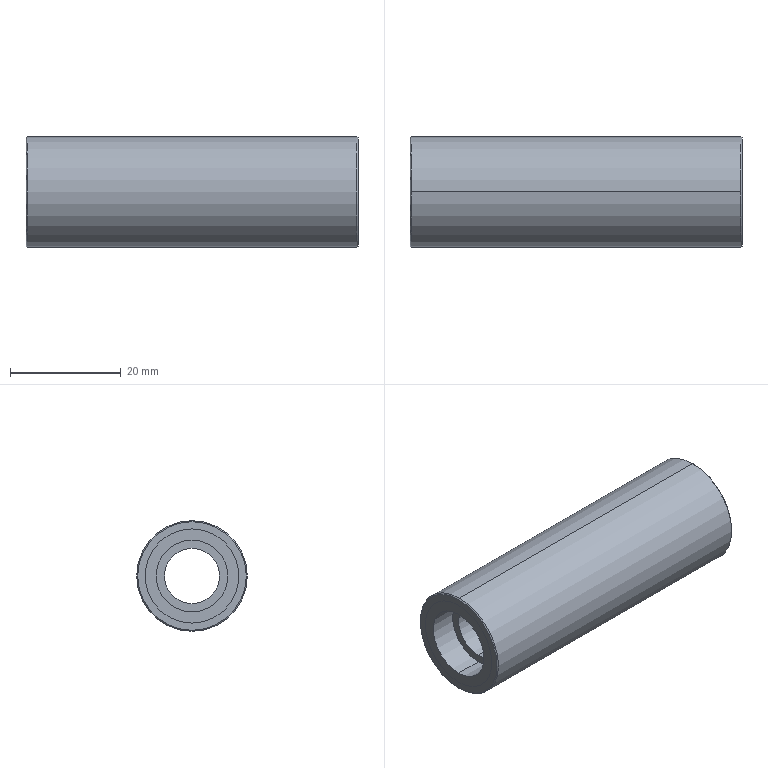Part | SolidWorks | features Chamfer 1, ICE 1, Revolution 1 | 2 solids | 22 faces | box 60 x 20 x 20 mm | volume 13593 mm3 | cylinder 12 | plane 6 | cone 4 | commonest cylinder face diameters 13 x4 17 x4 10 x2 20 x2
STEP:
#1=CARTESIAN_POINT('',(5.,0.,-6.5));
#2=VERTEX_POINT('',#1);
#3=CARTESIAN_POINT('',(5.,0.,6.5));
#4=VERTEX_POINT('',#3);
#5=CARTESIAN_POINT('',(5.,0.,0.));
#6=DIRECTION('',(-1.,0.,0.));
#7=DIRECTION('',(0.,0.,1.));
#8=AXIS2_PLACEMENT_3D('',#5,#6,#7);
#9=CIRCLE('',#8,6.5);
#10=EDGE_CURVE('',#2,#4,#9,.T.);
#11=ORIENTED_EDGE('',*,*,#10,.F.);
#12=CARTESIAN_POINT('',(0.,0.,-6.5));
#13=VERTEX_POINT('',#12);
#14=CARTESIAN_POINT('',(0.,0.,-6.5));
#15=DIRECTION('',(-1.,0.,0.));
#16=VECTOR('',#15,1000.);
#17=LINE('',#14,#16);
#18=EDGE_CURVE('',#2,#13,#17,.T.);
#19=ORIENTED_EDGE('',*,*,#18,.T.);
#20=CARTESIAN_POINT('',(0.,0.,6.5));
#21=VERTEX_POINT('',#20);
#22=CARTESIAN_POINT('',(0.,0.,0.));
#23=DIRECTION('',(-1.,0.,0.));
#24=DIRECTION('',(0.,0.,1.));
#25=AXIS2_PLACEMENT_3D('',#22,#23,#24);
#26=CIRCLE('',#25,6.5);
#27=EDGE_CURVE('',#13,#21,#26,.T.);
#28=ORIENTED_EDGE('',*,*,#27,.T.);
#29=CARTESIAN_POINT('',(0.,0.,6.5));
#30=DIRECTION('',(-1.,0.,0.));
#31=VECTOR('',#30,1000.);
#32=LINE('',#29,#31);
#33=EDGE_CURVE('',#4,#21,#32,.T.);
#34=ORIENTED_EDGE('',*,*,#33,.F.);
#35=EDGE_LOOP('',(#11,#19,#28,#34));
#36=FACE_OUTER_BOUND('',#35,.T.);
#37=CARTESIAN_POINT('',(0.,0.,0.));
#38=DIRECTION('',(-1.,0.,0.));
#39=DIRECTION('',(0.,0.,1.));
#40=AXIS2_PLACEMENT_3D('',#37,#38,#39);
#41=CYLINDRICAL_SURFACE('',#40,6.5);
#42=ADVANCED_FACE('',(#36),#41,.F.);
#43=CARTESIAN_POINT('',(55.,0.,-5.));
#44=VERTEX_POINT('',#43);
#45=CARTESIAN_POINT('',(55.,0.,5.));
#46=VERTEX_POINT('',#45);
#47=CARTESIAN_POINT('',(55.,0.,0.));
#48=DIRECTION('',(-1.,0.,0.));
#49=DIRECTION('',(0.,0.,1.));
#50=AXIS2_PLACEMENT_3D('',#47,#48,#49);
#51=CIRCLE('',#50,5.);
#52=EDGE_CURVE('',#44,#46,#51,.T.);
#53=ORIENTED_EDGE('',*,*,#52,.F.);
#54=CARTESIAN_POINT('',(5.,0.,-5.));
#55=VERTEX_POINT('',#54);
#56=CARTESIAN_POINT('',(0.,0.,-5.));
#57=DIRECTION('',(-1.,0.,0.));
#58=VECTOR('',#57,1000.);
#59=LINE('',#56,#58);
#60=EDGE_CURVE('',#44,#55,#59,.T.);
#61=ORIENTED_EDGE('',*,*,#60,.T.);
#62=CARTESIAN_POINT('',(5.,0.,5.));
#63=VERTEX_POINT('',#62);
#64=CARTESIAN_POINT('',(5.,0.,0.));
#65=DIRECTION('',(-1.,0.,0.));
#66=DIRECTION('',(0.,0.,1.));
#67=AXIS2_PLACEMENT_3D('',#64,#65,#66);
#68=CIRCLE('',#67,5.);
#69=EDGE_CURVE('',#55,#63,#68,.T.);
#70=ORIENTED_EDGE('',*,*,#69,.T.);
#71=CARTESIAN_POINT('',(0.,0.,5.));
#72=DIRECTION('',(-1.,0.,0.));
#73=VECTOR('',#72,1000.);
#74=LINE('',#71,#73);
#75=EDGE_CURVE('',#46,#63,#74,.T.);
#76=ORIENTED_EDGE('',*,*,#75,.F.);
#77=EDGE_LOOP('',(#53,#61,#70,#76));
#78=FACE_OUTER_BOUND('',#77,.T.);
#79=CARTESIAN_POINT('',(0.,0.,0.));
#80=DIRECTION('',(-1.,0.,0.));
#81=DIRECTION('',(0.,0.,1.));
#82=AXIS2_PLACEMENT_3D('',#79,#80,#81);
#83=CYLINDRICAL_SURFACE('',#82,5.);
#84=ADVANCED_FACE('',(#78),#83,.F.);
#85=CARTESIAN_POINT('',(60.,0.,-6.5));
#86=VERTEX_POINT('',#85);
#87=CARTESIAN_POINT('',(60.,0.,6.5));
#88=VERTEX_POINT('',#87);
#89=CARTESIAN_POINT('',(60.,0.,0.));
#90=DIRECTION('',(-1.,0.,0.));
#91=DIRECTION('',(0.,0.,1.));
#92=AXIS2_PLACEMENT_3D('',#89,#90,#91);
#93=CIRCLE('',#92,6.5);
#94=EDGE_CURVE('',#86,#88,#93,.T.);
#95=ORIENTED_EDGE('',*,*,#94,.F.);
#96=CARTESIAN_POINT('',(55.,0.,-6.5));
#97=VERTEX_POINT('',#96);
#98=CARTESIAN_POINT('',(0.,0.,-6.5));
#99=DIRECTION('',(-1.,0.,0.));
#100=VECTOR('',#99,1000.);
#101=LINE('',#98,#100);
#102=EDGE_CURVE('',#86,#97,#101,.T.);
#103=ORIENTED_EDGE('',*,*,#102,.T.);
#104=CARTESIAN_POINT('',(55.,0.,6.5));
#105=VERTEX_POINT('',#104);
#106=CARTESIAN_POINT('',(55.,0.,0.));
#107=DIRECTION('',(-1.,0.,0.));
#108=DIRECTION('',(0.,0.,1.));
#109=AXIS2_PLACEMENT_3D('',#106,#107,#108);
#110=CIRCLE('',#109,6.5);
#111=EDGE_CURVE('',#97,#105,#110,.T.);
#112=ORIENTED_EDGE('',*,*,#111,.T.);
#113=CARTESIAN_POINT('',(0.,0.,6.5));
#114=DIRECTION('',(-1.,0.,0.));
#115=VECTOR('',#114,1000.);
#116=LINE('',#113,#115);
#117=EDGE_CURVE('',#88,#105,#116,.T.);
#118=ORIENTED_EDGE('',*,*,#117,.F.);
#119=EDGE_LOOP('',(#95,#103,#112,#118));
#120=FACE_OUTER_BOUND('',#119,.T.);
#121=CARTESIAN_POINT('',(0.,0.,0.));
#122=DIRECTION('',(-1.,0.,0.));
#123=DIRECTION('',(0.,0.,1.));
#124=AXIS2_PLACEMENT_3D('',#121,#122,#123);
#125=CYLINDRICAL_SURFACE('',#124,6.5);
#126=ADVANCED_FACE('',(#120),#125,.F.);
#127=CARTESIAN_POINT('',(60.,0.,8.5));
#128=VERTEX_POINT('',#127);
#129=CARTESIAN_POINT('',(60.,0.,-8.5));
#130=VERTEX_POINT('',#129);
#131=CARTESIAN_POINT('',(60.,0.,0.));
#132=DIRECTION('',(-1.,0.,0.));
#133=DIRECTION('',(0.,0.,1.));
#134=AXIS2_PLACEMENT_3D('',#131,#132,#133);
#135=CIRCLE('',#134,8.5);
#136=EDGE_CURVE('',#128,#130,#135,.T.);
#137=ORIENTED_EDGE('',*,*,#136,.T.);
#138=CARTESIAN_POINT('',(0.,0.,-8.5));
#139=VERTEX_POINT('',#138);
#140=CARTESIAN_POINT('',(0.,0.,-8.5));
#141=DIRECTION('',(-1.,0.,0.));
#142=VECTOR('',#141,1000.);
#143=LINE('',#140,#142);
#144=EDGE_CURVE('',#130,#139,#143,.T.);
#145=ORIENTED_EDGE('',*,*,#144,.T.);
#146=CARTESIAN_POINT('',(0.,0.,8.5));
#147=VERTEX_POINT('',#146);
#148=CARTESIAN_POINT('',(0.,0.,0.));
#149=DIRECTION('',(-1.,0.,0.));
#150=DIRECTION('',(0.,0.,1.));
#151=AXIS2_PLACEMENT_3D('',#148,#149,#150);
#152=CIRCLE('',#151,8.5);
#153=EDGE_CURVE('',#147,#139,#152,.T.);
#154=ORIENTED_EDGE('',*,*,#153,.F.);
#155=CARTESIAN_POINT('',(0.,0.,8.5));
#156=DIRECTION('',(-1.,0.,0.));
#157=VECTOR('',#156,1000.);
#158=LINE('',#155,#157);
#159=EDGE_CURVE('',#128,#147,#158,.T.);
#160=ORIENTED_EDGE('',*,*,#159,.F.);
#161=EDGE_LOOP('',(#137,#145,#154,#160));
#162=FACE_OUTER_BOUND('',#161,.T.);
#163=CARTESIAN_POINT('',(0.,0.,0.));
#164=DIRECTION('',(-1.,0.,0.));
#165=DIRECTION('',(0.,0.,1.));
#166=AXIS2_PLACEMENT_3D('',#163,#164,#165);
#167=CYLINDRICAL_SURFACE('',#166,8.5);
#168=ADVANCED_FACE('',(#162),#167,.T.);
#169=CARTESIAN_POINT('',(0.,0.,0.));
#170=DIRECTION('',(-1.,0.,0.));
#171=DIRECTION('',(0.,0.,1.));
#172=AXIS2_PLACEMENT_3D('',#169,#170,#171);
#173=CIRCLE('',#172,6.5);
#174=EDGE_CURVE('',#21,#13,#173,.T.);
#175=ORIENTED_EDGE('',*,*,#174,.F.);
#176=ORIENTED_EDGE('',*,*,#27,.F.);
#177=EDGE_LOOP('',(#175,#176));
#178=FACE_BOUND('',#177,.T.);
#179=ORIENTED_EDGE('',*,*,#153,.T.);
#180=CARTESIAN_POINT('',(0.,0.,0.));
#181=DIRECTION('',(-1.,0.,0.));
#182=DIRECTION('',(0.,0.,1.));
#183=AXIS2_PLACEMENT_3D('',#180,#181,#182);
#184=CIRCLE('',#183,8.5);
#185=EDGE_CURVE('',#139,#147,#184,.T.);
#186=ORIENTED_EDGE('',*,*,#185,.T.);
#187=EDGE_LOOP('',(#179,#186));
#188=FACE_OUTER_BOUND('',#187,.T.);
#189=CARTESIAN_POINT('',(0.,6.5,0.));
#190=DIRECTION('',(1.,0.,0.));
#191=DIRECTION('',(0.,0.,-1.));
#192=AXIS2_PLACEMENT_3D('',#189,#190,#191);
#193=PLANE('',#192);
#194=ADVANCED_FACE('',(#178,#188),#193,.F.);
#195=ORIENTED_EDGE('',*,*,#144,.F.);
#196=CARTESIAN_POINT('',(60.,0.,0.));
#197=DIRECTION('',(-1.,0.,0.));
#198=DIRECTION('',(0.,0.,1.));
#199=AXIS2_PLACEMENT_3D('',#196,#197,#198);
#200=CIRCLE('',#199,8.5);
#201=EDGE_CURVE('',#130,#128,#200,.T.);
#202=ORIENTED_EDGE('',*,*,#201,.T.);
#203=ORIENTED_EDGE('',*,*,#159,.T.);
#204=ORIENTED_EDGE('',*,*,#185,.F.);
#205=EDGE_LOOP('',(#195,#202,#203,#204));
#206=FACE_OUTER_BOUND('',#205,.T.);
#207=CARTESIAN_POINT('',(0.,0.,0.));
#208=DIRECTION('',(-1.,0.,0.));
#209=DIRECTION('',(0.,0.,1.));
#210=AXIS2_PLACEMENT_3D('',#207,#208,#209);
#211=CYLINDRICAL_SURFACE('',#210,8.5);
#212=ADVANCED_FACE('',(#206),#211,.T.);
#213=ORIENTED_EDGE('',*,*,#136,.F.);
#214=ORIENTED_EDGE('',*,*,#201,.F.);
#215=EDGE_LOOP('',(#213,#214));
#216=FACE_OUTER_BOUND('',#215,.T.);
#217=CARTESIAN_POINT('',(60.,0.,0.));
#218=DIRECTION('',(-1.,0.,0.));
#219=DIRECTION('',(0.,0.,1.));
#220=AXIS2_PLACEMENT_3D('',#217,#218,#219);
#221=CIRCLE('',#220,6.5);
#222=EDGE_CURVE('',#88,#86,#221,.T.);
#223=ORIENTED_EDGE('',*,*,#222,.T.);
#224=ORIENTED_EDGE('',*,*,#94,.T.);
#225=EDGE_LOOP('',(#223,#224));
#226=FACE_BOUND('',#225,.T.);
#227=CARTESIAN_POINT('',(60.,8.5,0.));
#228=DIRECTION('',(-1.,0.,0.));
#229=DIRECTION('',(0.,0.,1.));
#230=AXIS2_PLACEMENT_3D('',#227,#228,#229);
#231=PLANE('',#230);
#232=ADVANCED_FACE('',(#216,#226),#231,.F.);
#233=ORIENTED_EDGE('',*,*,#102,.F.);
#234=ORIENTED_EDGE('',*,*,#222,.F.);
#235=ORIENTED_EDGE('',*,*,#117,.T.);
#236=CARTESIAN_POINT('',(55.,0.,0.));
#237=DIRECTION('',(-1.,0.,0.));
#238=DIRECTION('',(0.,0.,1.));
#239=AXIS2_PLACEMENT_3D('',#236,#237,#238);
#240=CIRCLE('',#239,6.5);
#241=EDGE_CURVE('',#105,#97,#240,.T.);
#242=ORIENTED_EDGE('',*,*,#241,.T.);
#243=EDGE_LOOP('',(#233,#234,#235,#242));
#244=FACE_OUTER_BOUND('',#243,.T.);
#245=CARTESIAN_POINT('',(0.,0.,0.));
#246=DIRECTION('',(-1.,0.,0.));
#247=DIRECTION('',(0.,0.,1.));
#248=AXIS2_PLACEMENT_3D('',#245,#246,#247);
#249=CYLINDRICAL_SURFACE('',#248,6.5);
#250=ADVANCED_FACE('',(#244),#249,.F.);
#251=ORIENTED_EDGE('',*,*,#241,.F.);
#252=ORIENTED_EDGE('',*,*,#111,.F.);
#253=EDGE_LOOP('',(#251,#252));
#254=FACE_OUTER_BOUND('',#253,.T.);
#255=CARTESIAN_POINT('',(55.,0.,0.));
#256=DIRECTION('',(-1.,0.,0.));
#257=DIRECTION('',(0.,0.,1.));
#258=AXIS2_PLACEMENT_3D('',#255,#256,#257);
#259=CIRCLE('',#258,5.);
#260=EDGE_CURVE('',#46,#44,#259,.T.);
#261=ORIENTED_EDGE('',*,*,#260,.T.);
#262=ORIENTED_EDGE('',*,*,#52,.T.);
#263=EDGE_LOOP('',(#261,#262));
#264=FACE_BOUND('',#263,.T.);
#265=CARTESIAN_POINT('',(55.,6.5,0.));
#266=DIRECTION('',(-1.,0.,0.));
#267=DIRECTION('',(0.,0.,1.));
#268=AXIS2_PLACEMENT_3D('',#265,#266,#267);
#269=PLANE('',#268);
#270=ADVANCED_FACE('',(#254,#264),#269,.F.);
#271=ORIENTED_EDGE('',*,*,#60,.F.);
#272=ORIENTED_EDGE('',*,*,#260,.F.);
#273=ORIENTED_EDGE('',*,*,#75,.T.);
#274=CARTESIAN_POINT('',(5.,0.,0.));
#275=DIRECTION('',(-1.,0.,0.));
#276=DIRECTION('',(0.,0.,1.));
#277=AXIS2_PLACEMENT_3D('',#274,#275,#276);
#278=CIRCLE('',#277,5.);
#279=EDGE_CURVE('',#63,#55,#278,.T.);
#280=ORIENTED_EDGE('',*,*,#279,.T.);
#281=EDGE_LOOP('',(#271,#272,#273,#280));
#282=FACE_OUTER_BOUND('',#281,.T.);
#283=CARTESIAN_POINT('',(0.,0.,0.));
#284=DIRECTION('',(-1.,0.,0.));
#285=DIRECTION('',(0.,0.,1.));
#286=AXIS2_PLACEMENT_3D('',#283,#284,#285);
#287=CYLINDRICAL_SURFACE('',#286,5.);
#288=ADVANCED_FACE('',(#282),#287,.F.);
#289=ORIENTED_EDGE('',*,*,#279,.F.);
#290=ORIENTED_EDGE('',*,*,#69,.F.);
#291=EDGE_LOOP('',(#289,#290));
#292=FACE_BOUND('',#291,.T.);
#293=CARTESIAN_POINT('',(5.,0.,0.));
#294=DIRECTION('',(-1.,0.,0.));
#295=DIRECTION('',(0.,0.,1.));
#296=AXIS2_PLACEMENT_3D('',#293,#294,#295);
#297=CIRCLE('',#296,6.5);
#298=EDGE_CURVE('',#4,#2,#297,.T.);
#299=ORIENTED_EDGE('',*,*,#298,.T.);
#300=ORIENTED_EDGE('',*,*,#10,.T.);
#301=EDGE_LOOP('',(#299,#300));
#302=FACE_OUTER_BOUND('',#301,.T.);
#303=CARTESIAN_POINT('',(5.,5.,0.));
#304=DIRECTION('',(1.,0.,0.));
#305=DIRECTION('',(0.,0.,-1.));
#306=AXIS2_PLACEMENT_3D('',#303,#304,#305);
#307=PLANE('',#306);
#308=ADVANCED_FACE('',(#292,#302),#307,.F.);
#309=ORIENTED_EDGE('',*,*,#18,.F.);
#310=ORIENTED_EDGE('',*,*,#298,.F.);
#311=ORIENTED_EDGE('',*,*,#33,.T.);
#312=ORIENTED_EDGE('',*,*,#174,.T.);
#313=EDGE_LOOP('',(#309,#310,#311,#312));
#314=FACE_OUTER_BOUND('',#313,.T.);
#315=CARTESIAN_POINT('',(0.,0.,0.));
#316=DIRECTION('',(-1.,0.,0.));
#317=DIRECTION('',(0.,0.,1.));
#318=AXIS2_PLACEMENT_3D('',#315,#316,#317);
#319=CYLINDRICAL_SURFACE('',#318,6.5);
#320=ADVANCED_FACE('',(#314),#319,.F.);
#321=CLOSED_SHELL('',(#42,#84,#126,#168,#194,#212,#232,#250,#270,#288,#308,#320));
#322=MANIFOLD_SOLID_BREP('',#321);
#323=CARTESIAN_POINT('',(60.,0.,-9.8));
#324=VERTEX_POINT('',#323);
#325=CARTESIAN_POINT('',(60.,0.,9.8));
#326=VERTEX_POINT('',#325);
#327=CARTESIAN_POINT('',(60.,0.,0.));
#328=DIRECTION('',(1.,0.,0.));
#329=DIRECTION('',(0.,0.,-1.));
#330=AXIS2_PLACEMENT_3D('',#327,#328,#329);
#331=CIRCLE('',#330,9.8);
#332=EDGE_CURVE('',#324,#326,#331,.T.);
#333=ORIENTED_EDGE('',*,*,#332,.F.);
#334=CARTESIAN_POINT('',(59.8,0.,-10.));
#335=VERTEX_POINT('',#334);
#336=CARTESIAN_POINT('',(60.,0.,-9.8));
#337=DIRECTION('',(-0.7071,0.,-0.7071));
#338=VECTOR('',#337,1000.);
#339=LINE('',#336,#338);
#340=EDGE_CURVE('',#324,#335,#339,.T.);
#341=ORIENTED_EDGE('',*,*,#340,.T.);
#342=CARTESIAN_POINT('',(59.8,0.,10.));
#343=VERTEX_POINT('',#342);
#344=CARTESIAN_POINT('',(59.8,0.,0.));
#345=DIRECTION('',(-1.,0.,0.));
#346=DIRECTION('',(0.,0.,-1.));
#347=AXIS2_PLACEMENT_3D('',#344,#345,#346);
#348=CIRCLE('',#347,10.);
#349=EDGE_CURVE('',#343,#335,#348,.T.);
#350=ORIENTED_EDGE('',*,*,#349,.F.);
#351=CARTESIAN_POINT('',(60.,0.,9.8));
#352=DIRECTION('',(-0.7071,0.,0.7071));
#353=VECTOR('',#352,1000.);
#354=LINE('',#351,#353);
#355=EDGE_CURVE('',#326,#343,#354,.T.);
#356=ORIENTED_EDGE('',*,*,#355,.F.);
#357=EDGE_LOOP('',(#333,#341,#350,#356));
#358=FACE_OUTER_BOUND('',#357,.T.);
#359=CARTESIAN_POINT('',(60.,0.,0.));
#360=DIRECTION('',(-1.,0.,0.));
#361=DIRECTION('',(0.,0.,1.));
#362=AXIS2_PLACEMENT_3D('',#359,#360,#361);
#363=CONICAL_SURFACE('',#362,9.8,0.7854);
#364=ADVANCED_FACE('',(#358),#363,.T.);
#365=CARTESIAN_POINT('',(0.,0.,9.8));
#366=VERTEX_POINT('',#365);
#367=CARTESIAN_POINT('',(0.,0.,-9.8));
#368=VERTEX_POINT('',#367);
#369=CARTESIAN_POINT('',(0.,0.,0.));
#370=DIRECTION('',(-1.,0.,0.));
#371=DIRECTION('',(0.,0.,-1.));
#372=AXIS2_PLACEMENT_3D('',#369,#370,#371);
#373=CIRCLE('',#372,9.8);
#374=EDGE_CURVE('',#366,#368,#373,.T.);
#375=ORIENTED_EDGE('',*,*,#374,.F.);
#376=CARTESIAN_POINT('',(0.2,0.,10.));
#377=VERTEX_POINT('',#376);
#378=CARTESIAN_POINT('',(0.,0.,9.8));
#379=DIRECTION('',(0.7071,0.,0.7071));
#380=VECTOR('',#379,1000.);
#381=LINE('',#378,#380);
#382=EDGE_CURVE('',#366,#377,#381,.T.);
#383=ORIENTED_EDGE('',*,*,#382,.T.);
#384=CARTESIAN_POINT('',(0.2,0.,-10.));
#385=VERTEX_POINT('',#384);
#386=CARTESIAN_POINT('',(0.2,0.,0.));
#387=DIRECTION('',(1.,0.,0.));
#388=DIRECTION('',(0.,0.,-1.));
#389=AXIS2_PLACEMENT_3D('',#386,#387,#388);
#390=CIRCLE('',#389,10.);
#391=EDGE_CURVE('',#385,#377,#390,.T.);
#392=ORIENTED_EDGE('',*,*,#391,.F.);
#393=CARTESIAN_POINT('',(0.,0.,-9.8));
#394=DIRECTION('',(0.7071,0.,-0.7071));
#395=VECTOR('',#394,1000.);
#396=LINE('',#393,#395);
#397=EDGE_CURVE('',#368,#385,#396,.T.);
#398=ORIENTED_EDGE('',*,*,#397,.F.);
#399=EDGE_LOOP('',(#375,#383,#392,#398));
#400=FACE_OUTER_BOUND('',#399,.T.);
#401=CARTESIAN_POINT('',(0.,0.,0.));
#402=DIRECTION('',(1.,0.,0.));
#403=DIRECTION('',(0.,0.,-1.));
#404=AXIS2_PLACEMENT_3D('',#401,#402,#403);
#405=CONICAL_SURFACE('',#404,9.8,0.7854);
#406=ADVANCED_FACE('',(#400),#405,.T.);
#407=CARTESIAN_POINT('',(0.,0.,-8.5));
#408=VERTEX_POINT('',#407);
#409=CARTESIAN_POINT('',(0.,0.,8.5));
#410=VERTEX_POINT('',#409);
#411=CARTESIAN_POINT('',(0.,0.,0.));
#412=DIRECTION('',(-1.,0.,0.));
#413=DIRECTION('',(0.,0.,-1.));
#414=AXIS2_PLACEMENT_3D('',#411,#412,#413);
#415=CIRCLE('',#414,8.5);
#416=EDGE_CURVE('',#408,#410,#415,.T.);
#417=ORIENTED_EDGE('',*,*,#416,.T.);
#418=CARTESIAN_POINT('',(60.,0.,8.5));
#419=VERTEX_POINT('',#418);
#420=CARTESIAN_POINT('',(-28.284,0.,8.5));
#421=DIRECTION('',(1.,0.,0.));
#422=VECTOR('',#421,1000.);
#423=LINE('',#420,#422);
#424=EDGE_CURVE('',#410,#419,#423,.T.);
#425=ORIENTED_EDGE('',*,*,#424,.T.);
#426=CARTESIAN_POINT('',(60.,0.,-8.5));
#427=VERTEX_POINT('',#426);
#428=CARTESIAN_POINT('',(60.,0.,0.));
#429=DIRECTION('',(1.,0.,0.));
#430=DIRECTION('',(0.,0.,-1.));
#431=AXIS2_PLACEMENT_3D('',#428,#429,#430);
#432=CIRCLE('',#431,8.5);
#433=EDGE_CURVE('',#419,#427,#432,.T.);
#434=ORIENTED_EDGE('',*,*,#433,.T.);
#435=CARTESIAN_POINT('',(-28.284,0.,-8.5));
#436=DIRECTION('',(1.,0.,0.));
#437=VECTOR('',#436,1000.);
#438=LINE('',#435,#437);
#439=EDGE_CURVE('',#408,#427,#438,.T.);
#440=ORIENTED_EDGE('',*,*,#439,.F.);
#441=EDGE_LOOP('',(#417,#425,#434,#440));
#442=FACE_OUTER_BOUND('',#441,.T.);
#443=CARTESIAN_POINT('',(-28.284,0.,0.));
#444=DIRECTION('',(1.,0.,0.));
#445=DIRECTION('',(0.,0.,-1.));
#446=AXIS2_PLACEMENT_3D('',#443,#444,#445);
#447=CYLINDRICAL_SURFACE('',#446,8.5);
#448=ADVANCED_FACE('',(#442),#447,.F.);
#449=ORIENTED_EDGE('',*,*,#391,.T.);
#450=CARTESIAN_POINT('',(-28.284,0.,10.));
#451=DIRECTION('',(1.,0.,0.));
#452=VECTOR('',#451,1000.);
#453=LINE('',#450,#452);
#454=EDGE_CURVE('',#377,#343,#453,.T.);
#455=ORIENTED_EDGE('',*,*,#454,.T.);
#456=ORIENTED_EDGE('',*,*,#349,.T.);
#457=CARTESIAN_POINT('',(-28.284,0.,-10.));
#458=DIRECTION('',(1.,0.,0.));
#459=VECTOR('',#458,1000.);
#460=LINE('',#457,#459);
#461=EDGE_CURVE('',#385,#335,#460,.T.);
#462=ORIENTED_EDGE('',*,*,#461,.F.);
#463=EDGE_LOOP('',(#449,#455,#456,#462));
#464=FACE_OUTER_BOUND('',#463,.T.);
#465=CARTESIAN_POINT('',(-28.284,0.,0.));
#466=DIRECTION('',(1.,0.,0.));
#467=DIRECTION('',(0.,0.,-1.));
#468=AXIS2_PLACEMENT_3D('',#465,#466,#467);
#469=CYLINDRICAL_SURFACE('',#468,10.);
#470=ADVANCED_FACE('',(#464),#469,.T.);
#471=ORIENTED_EDGE('',*,*,#454,.F.);
#472=CARTESIAN_POINT('',(0.2,0.,0.));
#473=DIRECTION('',(1.,0.,0.));
#474=DIRECTION('',(0.,0.,-1.));
#475=AXIS2_PLACEMENT_3D('',#472,#473,#474);
#476=CIRCLE('',#475,10.);
#477=EDGE_CURVE('',#377,#385,#476,.T.);
#478=ORIENTED_EDGE('',*,*,#477,.T.);
#479=ORIENTED_EDGE('',*,*,#461,.T.);
#480=CARTESIAN_POINT('',(59.8,0.,0.));
#481=DIRECTION('',(-1.,0.,0.));
#482=DIRECTION('',(0.,0.,-1.));
#483=AXIS2_PLACEMENT_3D('',#480,#481,#482);
#484=CIRCLE('',#483,10.);
#485=EDGE_CURVE('',#335,#343,#484,.T.);
#486=ORIENTED_EDGE('',*,*,#485,.T.);
#487=EDGE_LOOP('',(#471,#478,#479,#486));
#488=FACE_OUTER_BOUND('',#487,.T.);
#489=CARTESIAN_POINT('',(-28.284,0.,0.));
#490=DIRECTION('',(1.,0.,0.));
#491=DIRECTION('',(0.,0.,-1.));
#492=AXIS2_PLACEMENT_3D('',#489,#490,#491);
#493=CYLINDRICAL_SURFACE('',#492,10.);
#494=ADVANCED_FACE('',(#488),#493,.T.);
#495=CARTESIAN_POINT('',(60.,0.,0.));
#496=DIRECTION('',(1.,0.,0.));
#497=DIRECTION('',(0.,0.,-1.));
#498=AXIS2_PLACEMENT_3D('',#495,#496,#497);
#499=CIRCLE('',#498,9.8);
#500=EDGE_CURVE('',#326,#324,#499,.T.);
#501=ORIENTED_EDGE('',*,*,#500,.T.);
#502=ORIENTED_EDGE('',*,*,#332,.T.);
#503=EDGE_LOOP('',(#501,#502));
#504=FACE_OUTER_BOUND('',#503,.T.);
#505=CARTESIAN_POINT('',(60.,0.,0.));
#506=DIRECTION('',(1.,0.,0.));
#507=DIRECTION('',(0.,0.,-1.));
#508=AXIS2_PLACEMENT_3D('',#505,#506,#507);
#509=CIRCLE('',#508,8.5);
#510=EDGE_CURVE('',#427,#419,#509,.T.);
#511=ORIENTED_EDGE('',*,*,#510,.F.);
#512=ORIENTED_EDGE('',*,*,#433,.F.);
#513=EDGE_LOOP('',(#511,#512));
#514=FACE_BOUND('',#513,.T.);
#515=CARTESIAN_POINT('',(60.,0.,0.));
#516=DIRECTION('',(1.,0.,0.));
#517=DIRECTION('',(0.,0.,-1.));
#518=AXIS2_PLACEMENT_3D('',#515,#516,#517);
#519=PLANE('',#518);
#520=ADVANCED_FACE('',(#504,#514),#519,.T.);
#521=ORIENTED_EDGE('',*,*,#424,.F.);
#522=CARTESIAN_POINT('',(0.,0.,0.));
#523=DIRECTION('',(-1.,0.,0.));
#524=DIRECTION('',(0.,0.,-1.));
#525=AXIS2_PLACEMENT_3D('',#522,#523,#524);
#526=CIRCLE('',#525,8.5);
#527=EDGE_CURVE('',#410,#408,#526,.T.);
#528=ORIENTED_EDGE('',*,*,#527,.T.);
#529=ORIENTED_EDGE('',*,*,#439,.T.);
#530=ORIENTED_EDGE('',*,*,#510,.T.);
#531=EDGE_LOOP('',(#521,#528,#529,#530));
#532=FACE_OUTER_BOUND('',#531,.T.);
#533=CARTESIAN_POINT('',(-28.284,0.,0.));
#534=DIRECTION('',(1.,0.,0.));
#535=DIRECTION('',(0.,0.,-1.));
#536=AXIS2_PLACEMENT_3D('',#533,#534,#535);
#537=CYLINDRICAL_SURFACE('',#536,8.5);
#538=ADVANCED_FACE('',(#532),#537,.F.);
#539=CARTESIAN_POINT('',(0.,0.,0.));
#540=DIRECTION('',(-1.,0.,0.));
#541=DIRECTION('',(0.,0.,-1.));
#542=AXIS2_PLACEMENT_3D('',#539,#540,#541);
#543=CIRCLE('',#542,9.8);
#544=EDGE_CURVE('',#368,#366,#543,.T.);
#545=ORIENTED_EDGE('',*,*,#544,.T.);
#546=ORIENTED_EDGE('',*,*,#374,.T.);
#547=EDGE_LOOP('',(#545,#546));
#548=FACE_OUTER_BOUND('',#547,.T.);
#549=ORIENTED_EDGE('',*,*,#416,.F.);
#550=ORIENTED_EDGE('',*,*,#527,.F.);
#551=EDGE_LOOP('',(#549,#550));
#552=FACE_BOUND('',#551,.T.);
#553=CARTESIAN_POINT('',(0.,6.5,0.));
#554=DIRECTION('',(1.,0.,0.));
#555=DIRECTION('',(0.,0.,-1.));
#556=AXIS2_PLACEMENT_3D('',#553,#554,#555);
#557=PLANE('',#556);
#558=ADVANCED_FACE('',(#548,#552),#557,.F.);
#559=ORIENTED_EDGE('',*,*,#382,.F.);
#560=ORIENTED_EDGE('',*,*,#544,.F.);
#561=ORIENTED_EDGE('',*,*,#397,.T.);
#562=ORIENTED_EDGE('',*,*,#477,.F.);
#563=EDGE_LOOP('',(#559,#560,#561,#562));
#564=FACE_OUTER_BOUND('',#563,.T.);
#565=CARTESIAN_POINT('',(0.,0.,0.));
#566=DIRECTION('',(1.,0.,0.));
#567=DIRECTION('',(0.,0.,-1.));
#568=AXIS2_PLACEMENT_3D('',#565,#566,#567);
#569=CONICAL_SURFACE('',#568,9.8,0.7854);
#570=ADVANCED_FACE('',(#564),#569,.T.);
#571=ORIENTED_EDGE('',*,*,#340,.F.);
#572=ORIENTED_EDGE('',*,*,#500,.F.);
#573=ORIENTED_EDGE('',*,*,#355,.T.);
#574=ORIENTED_EDGE('',*,*,#485,.F.);
#575=EDGE_LOOP('',(#571,#572,#573,#574));
#576=FACE_OUTER_BOUND('',#575,.T.);
#577=CARTESIAN_POINT('',(60.,0.,0.));
#578=DIRECTION('',(-1.,0.,0.));
#579=DIRECTION('',(0.,0.,1.));
#580=AXIS2_PLACEMENT_3D('',#577,#578,#579);
#581=CONICAL_SURFACE('',#580,9.8,0.7854);
#582=ADVANCED_FACE('',(#576),#581,.T.);
#583=CLOSED_SHELL('',(#364,#406,#448,#470,#494,#520,#538,#558,#570,#582));
#584=MANIFOLD_SOLID_BREP('',#583);
#585=CARTESIAN_POINT('',(0.,0.,0.));
#586=DIRECTION('',(0.,0.,1.));
#587=DIRECTION('',(1.,0.,0.));
#588=AXIS2_PLACEMENT_3D('',#585,#586,#587);
#589=(LENGTH_UNIT()NAMED_UNIT(*)SI_UNIT(.MILLI.,.METRE.));
#590=UNCERTAINTY_MEASURE_WITH_UNIT(LENGTH_MEASURE(0.00001),#589,'','');
#591=(NAMED_UNIT(*)PLANE_ANGLE_UNIT()SI_UNIT($,.RADIAN.));
#592=(NAMED_UNIT(*)SI_UNIT($,.STERADIAN.)SOLID_ANGLE_UNIT());
#593=(GEOMETRIC_REPRESENTATION_CONTEXT(3)GLOBAL_UNCERTAINTY_ASSIGNED_CONTEXT((#590))GLOBAL_UNIT_ASSIGNED_CONTEXT((#589,#591,#592))REPRESENTATION_CONTEXT('',''));
#594=ADVANCED_BREP_SHAPE_REPRESENTATION('',(#322,#584,#588),#593);